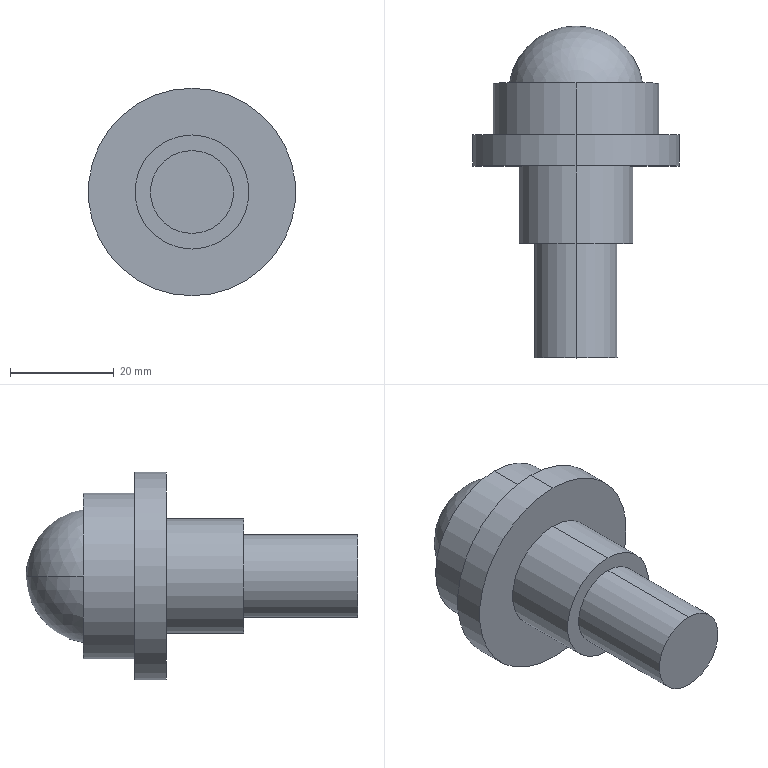Part | SolidWorks | features ICE 2, Revolution 1 | 1 solid | 15 faces | box 40 x 64 x 40 mm | volume 29255 mm3 | cylinder 8 | plane 5 | sphere 2 | commonest cylinder face diameters 16 x2 22 x2 32 x2 40 x2
STEP:
#1=CARTESIAN_POINT('',(0.,-37.,-8.));
#2=VERTEX_POINT('',#1);
#3=CARTESIAN_POINT('',(0.,-37.,8.));
#4=VERTEX_POINT('',#3);
#5=CARTESIAN_POINT('',(0.,-37.,0.));
#6=DIRECTION('',(0.,-1.,0.));
#7=DIRECTION('',(0.,0.,-1.));
#8=AXIS2_PLACEMENT_3D('',#5,#6,#7);
#9=CIRCLE('',#8,8.);
#10=EDGE_CURVE('',#2,#4,#9,.T.);
#11=ORIENTED_EDGE('',*,*,#10,.F.);
#12=CARTESIAN_POINT('',(0.,-15.,-8.));
#13=VERTEX_POINT('',#12);
#14=CARTESIAN_POINT('',(0.,-37.,-8.));
#15=DIRECTION('',(0.,1.,0.));
#16=VECTOR('',#15,1000.);
#17=LINE('',#14,#16);
#18=EDGE_CURVE('',#2,#13,#17,.T.);
#19=ORIENTED_EDGE('',*,*,#18,.T.);
#20=CARTESIAN_POINT('',(0.,-15.,8.));
#21=VERTEX_POINT('',#20);
#22=CARTESIAN_POINT('',(0.,-15.,0.));
#23=DIRECTION('',(0.,-1.,0.));
#24=DIRECTION('',(0.,0.,-1.));
#25=AXIS2_PLACEMENT_3D('',#22,#23,#24);
#26=CIRCLE('',#25,8.);
#27=EDGE_CURVE('',#13,#21,#26,.T.);
#28=ORIENTED_EDGE('',*,*,#27,.T.);
#29=CARTESIAN_POINT('',(0.,-37.,8.));
#30=DIRECTION('',(0.,1.,0.));
#31=VECTOR('',#30,1000.);
#32=LINE('',#29,#31);
#33=EDGE_CURVE('',#4,#21,#32,.T.);
#34=ORIENTED_EDGE('',*,*,#33,.F.);
#35=EDGE_LOOP('',(#11,#19,#28,#34));
#36=FACE_OUTER_BOUND('',#35,.T.);
#37=CARTESIAN_POINT('',(0.,-37.,0.));
#38=DIRECTION('',(0.,1.,0.));
#39=DIRECTION('',(0.,0.,1.));
#40=AXIS2_PLACEMENT_3D('',#37,#38,#39);
#41=CYLINDRICAL_SURFACE('',#40,8.);
#42=ADVANCED_FACE('',(#36),#41,.T.);
#43=CARTESIAN_POINT('',(0.,-15.,-11.));
#44=VERTEX_POINT('',#43);
#45=CARTESIAN_POINT('',(0.,-15.,11.));
#46=VERTEX_POINT('',#45);
#47=CARTESIAN_POINT('',(0.,-15.,0.));
#48=DIRECTION('',(0.,-1.,0.));
#49=DIRECTION('',(0.,0.,-1.));
#50=AXIS2_PLACEMENT_3D('',#47,#48,#49);
#51=CIRCLE('',#50,11.);
#52=EDGE_CURVE('',#44,#46,#51,.T.);
#53=ORIENTED_EDGE('',*,*,#52,.F.);
#54=CARTESIAN_POINT('',(0.,0.,-11.));
#55=VERTEX_POINT('',#54);
#56=CARTESIAN_POINT('',(0.,-15.,-11.));
#57=DIRECTION('',(0.,1.,0.));
#58=VECTOR('',#57,1000.);
#59=LINE('',#56,#58);
#60=EDGE_CURVE('',#44,#55,#59,.T.);
#61=ORIENTED_EDGE('',*,*,#60,.T.);
#62=CARTESIAN_POINT('',(0.,0.,11.));
#63=VERTEX_POINT('',#62);
#64=CARTESIAN_POINT('',(0.,0.,0.));
#65=DIRECTION('',(0.,-1.,0.));
#66=DIRECTION('',(0.,0.,-1.));
#67=AXIS2_PLACEMENT_3D('',#64,#65,#66);
#68=CIRCLE('',#67,11.);
#69=EDGE_CURVE('',#55,#63,#68,.T.);
#70=ORIENTED_EDGE('',*,*,#69,.T.);
#71=CARTESIAN_POINT('',(0.,-15.,11.));
#72=DIRECTION('',(0.,1.,0.));
#73=VECTOR('',#72,1000.);
#74=LINE('',#71,#73);
#75=EDGE_CURVE('',#46,#63,#74,.T.);
#76=ORIENTED_EDGE('',*,*,#75,.F.);
#77=EDGE_LOOP('',(#53,#61,#70,#76));
#78=FACE_OUTER_BOUND('',#77,.T.);
#79=CARTESIAN_POINT('',(0.,-15.,0.));
#80=DIRECTION('',(0.,1.,0.));
#81=DIRECTION('',(0.,0.,1.));
#82=AXIS2_PLACEMENT_3D('',#79,#80,#81);
#83=CYLINDRICAL_SURFACE('',#82,11.);
#84=ADVANCED_FACE('',(#78),#83,.T.);
#85=CARTESIAN_POINT('',(0.,6.,-20.));
#86=VERTEX_POINT('',#85);
#87=CARTESIAN_POINT('',(0.,6.,20.));
#88=VERTEX_POINT('',#87);
#89=CARTESIAN_POINT('',(0.,6.,0.));
#90=DIRECTION('',(0.,-1.,0.));
#91=DIRECTION('',(0.,0.,-1.));
#92=AXIS2_PLACEMENT_3D('',#89,#90,#91);
#93=CIRCLE('',#92,20.);
#94=EDGE_CURVE('',#86,#88,#93,.T.);
#95=ORIENTED_EDGE('',*,*,#94,.T.);
#96=CARTESIAN_POINT('',(0.,0.,20.));
#97=VERTEX_POINT('',#96);
#98=CARTESIAN_POINT('',(0.,0.,20.));
#99=DIRECTION('',(0.,-1.,0.));
#100=VECTOR('',#99,1000.);
#101=LINE('',#98,#100);
#102=EDGE_CURVE('',#88,#97,#101,.T.);
#103=ORIENTED_EDGE('',*,*,#102,.T.);
#104=CARTESIAN_POINT('',(0.,0.,-20.));
#105=VERTEX_POINT('',#104);
#106=CARTESIAN_POINT('',(0.,0.,0.));
#107=DIRECTION('',(0.,-1.,0.));
#108=DIRECTION('',(0.,0.,-1.));
#109=AXIS2_PLACEMENT_3D('',#106,#107,#108);
#110=CIRCLE('',#109,20.);
#111=EDGE_CURVE('',#105,#97,#110,.T.);
#112=ORIENTED_EDGE('',*,*,#111,.F.);
#113=CARTESIAN_POINT('',(0.,0.,-20.));
#114=DIRECTION('',(0.,-1.,0.));
#115=VECTOR('',#114,1000.);
#116=LINE('',#113,#115);
#117=EDGE_CURVE('',#86,#105,#116,.T.);
#118=ORIENTED_EDGE('',*,*,#117,.F.);
#119=EDGE_LOOP('',(#95,#103,#112,#118));
#120=FACE_OUTER_BOUND('',#119,.T.);
#121=CARTESIAN_POINT('',(0.,0.,0.));
#122=DIRECTION('',(0.,-1.,0.));
#123=DIRECTION('',(0.,0.,-1.));
#124=AXIS2_PLACEMENT_3D('',#121,#122,#123);
#125=CYLINDRICAL_SURFACE('',#124,20.);
#126=ADVANCED_FACE('',(#120),#125,.T.);
#127=CARTESIAN_POINT('',(0.,16.,-16.));
#128=VERTEX_POINT('',#127);
#129=CARTESIAN_POINT('',(0.,16.,16.));
#130=VERTEX_POINT('',#129);
#131=CARTESIAN_POINT('',(0.,16.,0.));
#132=DIRECTION('',(0.,-1.,0.));
#133=DIRECTION('',(0.,0.,-1.));
#134=AXIS2_PLACEMENT_3D('',#131,#132,#133);
#135=CIRCLE('',#134,16.);
#136=EDGE_CURVE('',#128,#130,#135,.T.);
#137=ORIENTED_EDGE('',*,*,#136,.T.);
#138=CARTESIAN_POINT('',(0.,6.,16.));
#139=VERTEX_POINT('',#138);
#140=CARTESIAN_POINT('',(0.,0.,16.));
#141=DIRECTION('',(0.,-1.,0.));
#142=VECTOR('',#141,1000.);
#143=LINE('',#140,#142);
#144=EDGE_CURVE('',#130,#139,#143,.T.);
#145=ORIENTED_EDGE('',*,*,#144,.T.);
#146=CARTESIAN_POINT('',(0.,6.,-16.));
#147=VERTEX_POINT('',#146);
#148=CARTESIAN_POINT('',(0.,6.,0.));
#149=DIRECTION('',(0.,-1.,0.));
#150=DIRECTION('',(0.,0.,-1.));
#151=AXIS2_PLACEMENT_3D('',#148,#149,#150);
#152=CIRCLE('',#151,16.);
#153=EDGE_CURVE('',#147,#139,#152,.T.);
#154=ORIENTED_EDGE('',*,*,#153,.F.);
#155=CARTESIAN_POINT('',(0.,0.,-16.));
#156=DIRECTION('',(0.,-1.,0.));
#157=VECTOR('',#156,1000.);
#158=LINE('',#155,#157);
#159=EDGE_CURVE('',#128,#147,#158,.T.);
#160=ORIENTED_EDGE('',*,*,#159,.F.);
#161=EDGE_LOOP('',(#137,#145,#154,#160));
#162=FACE_OUTER_BOUND('',#161,.T.);
#163=CARTESIAN_POINT('',(0.,0.,0.));
#164=DIRECTION('',(0.,-1.,0.));
#165=DIRECTION('',(0.,0.,-1.));
#166=AXIS2_PLACEMENT_3D('',#163,#164,#165);
#167=CYLINDRICAL_SURFACE('',#166,16.);
#168=ADVANCED_FACE('',(#162),#167,.T.);
#169=CARTESIAN_POINT('',(0.,27.,0.));
#170=VERTEX_POINT('',#169);
#171=CARTESIAN_POINT('',(12.845,16.,0.));
#172=VERTEX_POINT('',#171);
#173=CARTESIAN_POINT('',(0.,14.,0.));
#174=DIRECTION('',(0.,0.,-1.));
#175=DIRECTION('',(-1.,0.,0.));
#176=AXIS2_PLACEMENT_3D('',#173,#174,#175);
#177=CIRCLE('',#176,13.);
#178=EDGE_CURVE('',#170,#172,#177,.T.);
#179=ORIENTED_EDGE('',*,*,#178,.F.);
#180=CARTESIAN_POINT('',(-12.845,16.,0.));
#181=VERTEX_POINT('',#180);
#182=CARTESIAN_POINT('',(0.,14.,0.));
#183=DIRECTION('',(0.,0.,1.));
#184=DIRECTION('',(1.,0.,0.));
#185=AXIS2_PLACEMENT_3D('',#182,#183,#184);
#186=CIRCLE('',#185,13.);
#187=EDGE_CURVE('',#170,#181,#186,.T.);
#188=ORIENTED_EDGE('',*,*,#187,.T.);
#189=CARTESIAN_POINT('',(0.,16.,0.));
#190=DIRECTION('',(0.,-1.,0.));
#191=DIRECTION('',(0.,0.,-1.));
#192=AXIS2_PLACEMENT_3D('',#189,#190,#191);
#193=CIRCLE('',#192,12.845);
#194=EDGE_CURVE('',#172,#181,#193,.T.);
#195=ORIENTED_EDGE('',*,*,#194,.F.);
#196=EDGE_LOOP('',(#179,#188,#195));
#197=FACE_OUTER_BOUND('',#196,.T.);
#198=CARTESIAN_POINT('',(0.,14.,0.));
#199=DIRECTION('',(0.,0.,1.));
#200=DIRECTION('',(1.,0.,0.));
#201=AXIS2_PLACEMENT_3D('',#198,#199,#200);
#202=SPHERICAL_SURFACE('',#201,13.);
#203=ADVANCED_FACE('',(#197),#202,.T.);
#204=ORIENTED_EDGE('',*,*,#187,.F.);
#205=ORIENTED_EDGE('',*,*,#178,.T.);
#206=CARTESIAN_POINT('',(0.,16.,0.));
#207=DIRECTION('',(0.,-1.,0.));
#208=DIRECTION('',(0.,0.,-1.));
#209=AXIS2_PLACEMENT_3D('',#206,#207,#208);
#210=CIRCLE('',#209,12.845);
#211=EDGE_CURVE('',#181,#172,#210,.T.);
#212=ORIENTED_EDGE('',*,*,#211,.F.);
#213=EDGE_LOOP('',(#204,#205,#212));
#214=FACE_OUTER_BOUND('',#213,.T.);
#215=CARTESIAN_POINT('',(0.,14.,0.));
#216=DIRECTION('',(0.,0.,1.));
#217=DIRECTION('',(1.,0.,0.));
#218=AXIS2_PLACEMENT_3D('',#215,#216,#217);
#219=SPHERICAL_SURFACE('',#218,13.);
#220=ADVANCED_FACE('',(#214),#219,.T.);
#221=ORIENTED_EDGE('',*,*,#136,.F.);
#222=CARTESIAN_POINT('',(0.,16.,0.));
#223=DIRECTION('',(0.,-1.,0.));
#224=DIRECTION('',(0.,0.,-1.));
#225=AXIS2_PLACEMENT_3D('',#222,#223,#224);
#226=CIRCLE('',#225,16.);
#227=EDGE_CURVE('',#130,#128,#226,.T.);
#228=ORIENTED_EDGE('',*,*,#227,.F.);
#229=EDGE_LOOP('',(#221,#228));
#230=FACE_OUTER_BOUND('',#229,.T.);
#231=ORIENTED_EDGE('',*,*,#194,.T.);
#232=ORIENTED_EDGE('',*,*,#211,.T.);
#233=EDGE_LOOP('',(#231,#232));
#234=FACE_BOUND('',#233,.T.);
#235=CARTESIAN_POINT('',(-12.845,16.,0.));
#236=DIRECTION('',(0.,-1.,0.));
#237=DIRECTION('',(0.,0.,-1.));
#238=AXIS2_PLACEMENT_3D('',#235,#236,#237);
#239=PLANE('',#238);
#240=ADVANCED_FACE('',(#230,#234),#239,.F.);
#241=ORIENTED_EDGE('',*,*,#144,.F.);
#242=ORIENTED_EDGE('',*,*,#227,.T.);
#243=ORIENTED_EDGE('',*,*,#159,.T.);
#244=CARTESIAN_POINT('',(0.,6.,0.));
#245=DIRECTION('',(0.,-1.,0.));
#246=DIRECTION('',(0.,0.,-1.));
#247=AXIS2_PLACEMENT_3D('',#244,#245,#246);
#248=CIRCLE('',#247,16.);
#249=EDGE_CURVE('',#139,#147,#248,.T.);
#250=ORIENTED_EDGE('',*,*,#249,.F.);
#251=EDGE_LOOP('',(#241,#242,#243,#250));
#252=FACE_OUTER_BOUND('',#251,.T.);
#253=CARTESIAN_POINT('',(0.,0.,0.));
#254=DIRECTION('',(0.,-1.,0.));
#255=DIRECTION('',(0.,0.,-1.));
#256=AXIS2_PLACEMENT_3D('',#253,#254,#255);
#257=CYLINDRICAL_SURFACE('',#256,16.);
#258=ADVANCED_FACE('',(#252),#257,.T.);
#259=ORIENTED_EDGE('',*,*,#94,.F.);
#260=CARTESIAN_POINT('',(0.,6.,0.));
#261=DIRECTION('',(0.,-1.,0.));
#262=DIRECTION('',(0.,0.,-1.));
#263=AXIS2_PLACEMENT_3D('',#260,#261,#262);
#264=CIRCLE('',#263,20.);
#265=EDGE_CURVE('',#88,#86,#264,.T.);
#266=ORIENTED_EDGE('',*,*,#265,.F.);
#267=EDGE_LOOP('',(#259,#266));
#268=FACE_OUTER_BOUND('',#267,.T.);
#269=ORIENTED_EDGE('',*,*,#153,.T.);
#270=ORIENTED_EDGE('',*,*,#249,.T.);
#271=EDGE_LOOP('',(#269,#270));
#272=FACE_BOUND('',#271,.T.);
#273=CARTESIAN_POINT('',(-16.,6.,0.));
#274=DIRECTION('',(0.,-1.,0.));
#275=DIRECTION('',(0.,0.,-1.));
#276=AXIS2_PLACEMENT_3D('',#273,#274,#275);
#277=PLANE('',#276);
#278=ADVANCED_FACE('',(#268,#272),#277,.F.);
#279=ORIENTED_EDGE('',*,*,#102,.F.);
#280=ORIENTED_EDGE('',*,*,#265,.T.);
#281=ORIENTED_EDGE('',*,*,#117,.T.);
#282=CARTESIAN_POINT('',(0.,0.,0.));
#283=DIRECTION('',(0.,-1.,0.));
#284=DIRECTION('',(0.,0.,-1.));
#285=AXIS2_PLACEMENT_3D('',#282,#283,#284);
#286=CIRCLE('',#285,20.);
#287=EDGE_CURVE('',#97,#105,#286,.T.);
#288=ORIENTED_EDGE('',*,*,#287,.F.);
#289=EDGE_LOOP('',(#279,#280,#281,#288));
#290=FACE_OUTER_BOUND('',#289,.T.);
#291=CARTESIAN_POINT('',(0.,0.,0.));
#292=DIRECTION('',(0.,-1.,0.));
#293=DIRECTION('',(0.,0.,-1.));
#294=AXIS2_PLACEMENT_3D('',#291,#292,#293);
#295=CYLINDRICAL_SURFACE('',#294,20.);
#296=ADVANCED_FACE('',(#290),#295,.T.);
#297=CARTESIAN_POINT('',(0.,0.,0.));
#298=DIRECTION('',(0.,-1.,0.));
#299=DIRECTION('',(0.,0.,-1.));
#300=AXIS2_PLACEMENT_3D('',#297,#298,#299);
#301=CIRCLE('',#300,11.);
#302=EDGE_CURVE('',#63,#55,#301,.T.);
#303=ORIENTED_EDGE('',*,*,#302,.F.);
#304=ORIENTED_EDGE('',*,*,#69,.F.);
#305=EDGE_LOOP('',(#303,#304));
#306=FACE_BOUND('',#305,.T.);
#307=ORIENTED_EDGE('',*,*,#111,.T.);
#308=ORIENTED_EDGE('',*,*,#287,.T.);
#309=EDGE_LOOP('',(#307,#308));
#310=FACE_OUTER_BOUND('',#309,.T.);
#311=CARTESIAN_POINT('',(-20.,0.,0.));
#312=DIRECTION('',(0.,1.,0.));
#313=DIRECTION('',(0.,0.,1.));
#314=AXIS2_PLACEMENT_3D('',#311,#312,#313);
#315=PLANE('',#314);
#316=ADVANCED_FACE('',(#306,#310),#315,.F.);
#317=ORIENTED_EDGE('',*,*,#60,.F.);
#318=CARTESIAN_POINT('',(0.,-15.,0.));
#319=DIRECTION('',(0.,-1.,0.));
#320=DIRECTION('',(0.,0.,-1.));
#321=AXIS2_PLACEMENT_3D('',#318,#319,#320);
#322=CIRCLE('',#321,11.);
#323=EDGE_CURVE('',#46,#44,#322,.T.);
#324=ORIENTED_EDGE('',*,*,#323,.F.);
#325=ORIENTED_EDGE('',*,*,#75,.T.);
#326=ORIENTED_EDGE('',*,*,#302,.T.);
#327=EDGE_LOOP('',(#317,#324,#325,#326));
#328=FACE_OUTER_BOUND('',#327,.T.);
#329=CARTESIAN_POINT('',(0.,-15.,0.));
#330=DIRECTION('',(0.,1.,0.));
#331=DIRECTION('',(0.,0.,1.));
#332=AXIS2_PLACEMENT_3D('',#329,#330,#331);
#333=CYLINDRICAL_SURFACE('',#332,11.);
#334=ADVANCED_FACE('',(#328),#333,.T.);
#335=CARTESIAN_POINT('',(0.,-15.,0.));
#336=DIRECTION('',(0.,-1.,0.));
#337=DIRECTION('',(0.,0.,-1.));
#338=AXIS2_PLACEMENT_3D('',#335,#336,#337);
#339=CIRCLE('',#338,8.);
#340=EDGE_CURVE('',#21,#13,#339,.T.);
#341=ORIENTED_EDGE('',*,*,#340,.F.);
#342=ORIENTED_EDGE('',*,*,#27,.F.);
#343=EDGE_LOOP('',(#341,#342));
#344=FACE_BOUND('',#343,.T.);
#345=ORIENTED_EDGE('',*,*,#323,.T.);
#346=ORIENTED_EDGE('',*,*,#52,.T.);
#347=EDGE_LOOP('',(#345,#346));
#348=FACE_OUTER_BOUND('',#347,.T.);
#349=CARTESIAN_POINT('',(0.,-15.,0.));
#350=DIRECTION('',(0.,-1.,0.));
#351=DIRECTION('',(0.,0.,-1.));
#352=AXIS2_PLACEMENT_3D('',#349,#350,#351);
#353=PLANE('',#352);
#354=ADVANCED_FACE('',(#344,#348),#353,.T.);
#355=ORIENTED_EDGE('',*,*,#18,.F.);
#356=CARTESIAN_POINT('',(0.,-37.,0.));
#357=DIRECTION('',(0.,-1.,0.));
#358=DIRECTION('',(0.,0.,-1.));
#359=AXIS2_PLACEMENT_3D('',#356,#357,#358);
#360=CIRCLE('',#359,8.);
#361=EDGE_CURVE('',#4,#2,#360,.T.);
#362=ORIENTED_EDGE('',*,*,#361,.F.);
#363=ORIENTED_EDGE('',*,*,#33,.T.);
#364=ORIENTED_EDGE('',*,*,#340,.T.);
#365=EDGE_LOOP('',(#355,#362,#363,#364));
#366=FACE_OUTER_BOUND('',#365,.T.);
#367=CARTESIAN_POINT('',(0.,-37.,0.));
#368=DIRECTION('',(0.,1.,0.));
#369=DIRECTION('',(0.,0.,1.));
#370=AXIS2_PLACEMENT_3D('',#367,#368,#369);
#371=CYLINDRICAL_SURFACE('',#370,8.);
#372=ADVANCED_FACE('',(#366),#371,.T.);
#373=ORIENTED_EDGE('',*,*,#361,.T.);
#374=ORIENTED_EDGE('',*,*,#10,.T.);
#375=EDGE_LOOP('',(#373,#374));
#376=FACE_OUTER_BOUND('',#375,.T.);
#377=CARTESIAN_POINT('',(0.,-37.,0.));
#378=DIRECTION('',(0.,-1.,0.));
#379=DIRECTION('',(0.,0.,-1.));
#380=AXIS2_PLACEMENT_3D('',#377,#378,#379);
#381=PLANE('',#380);
#382=ADVANCED_FACE('',(#376),#381,.T.);
#383=CLOSED_SHELL('',(#42,#84,#126,#168,#203,#220,#240,#258,#278,#296,#316,#334,#354,#372,#382));
#384=MANIFOLD_SOLID_BREP('',#383);
#385=CARTESIAN_POINT('',(0.,0.,0.));
#386=DIRECTION('',(0.,0.,1.));
#387=DIRECTION('',(1.,0.,0.));
#388=AXIS2_PLACEMENT_3D('',#385,#386,#387);
#389=(LENGTH_UNIT()NAMED_UNIT(*)SI_UNIT(.MILLI.,.METRE.));
#390=UNCERTAINTY_MEASURE_WITH_UNIT(LENGTH_MEASURE(0.00001),#389,'','');
#391=(NAMED_UNIT(*)PLANE_ANGLE_UNIT()SI_UNIT($,.RADIAN.));
#392=(NAMED_UNIT(*)SI_UNIT($,.STERADIAN.)SOLID_ANGLE_UNIT());
#393=(GEOMETRIC_REPRESENTATION_CONTEXT(3)GLOBAL_UNCERTAINTY_ASSIGNED_CONTEXT((#390))GLOBAL_UNIT_ASSIGNED_CONTEXT((#389,#391,#392))REPRESENTATION_CONTEXT('',''));
#394=ADVANCED_BREP_SHAPE_REPRESENTATION('',(#384,#388),#393);